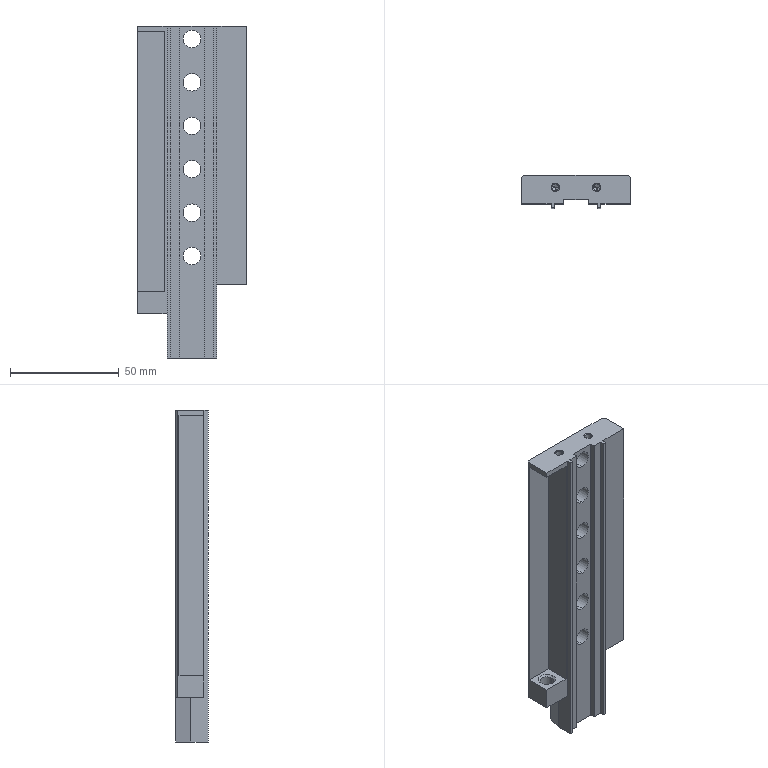Part | STEP file | 1 solid | 105 faces | box 50 x 15 x 153 mm | volume 64725 mm3 | plane 38 | cylinder 37 | cone 30 | commonest cylinder face diameters 3.2 x16 8 x14 5 x5 6.4 x2